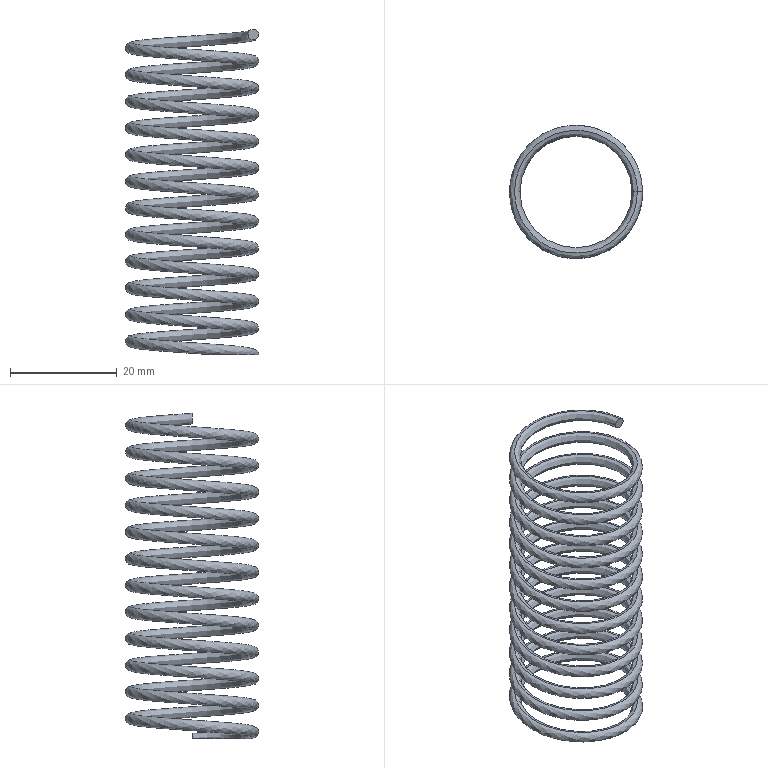Part | SolidWorks | features Helix 1, ICE 1, Sweep 1 | 1 solid | 5 faces | box 25 x 25 x 61 mm | volume 2708 mm3 | plane 3 | spline 2